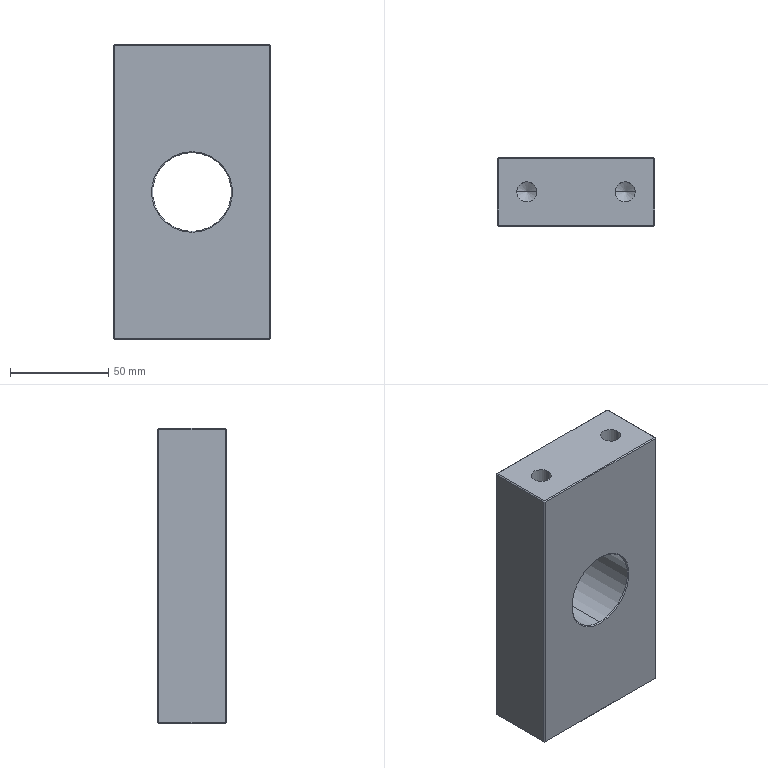Part | SolidWorks | features HoleWzd 2, Chamfer 1, Extrusion 1 | 1 solid | 48 faces | box 80 x 35 x 150 mm | volume 365960 mm3 | plane 26 | cone 12 | cylinder 10 | commonest cylinder face diameters 10.2 x8 40 x2
STEP:
#1=CARTESIAN_POINT('',(30.1,17.5,-45.75));
#2=VERTEX_POINT('',#1);
#3=CARTESIAN_POINT('',(19.9,17.5,-45.75));
#4=VERTEX_POINT('',#3);
#5=CARTESIAN_POINT('',(25.,17.5,-45.75));
#6=DIRECTION('',(0.,0.,-1.));
#7=DIRECTION('',(-1.,0.,0.));
#8=AXIS2_PLACEMENT_3D('',#5,#6,#7);
#9=CIRCLE('',#8,5.1);
#10=EDGE_CURVE('',#2,#4,#9,.T.);
#11=ORIENTED_EDGE('',*,*,#10,.F.);
#12=CARTESIAN_POINT('',(30.1,17.5,-75.));
#13=VERTEX_POINT('',#12);
#14=CARTESIAN_POINT('',(30.1,17.5,-75.));
#15=DIRECTION('',(0.,0.,-1.));
#16=VECTOR('',#15,1000.);
#17=LINE('',#14,#16);
#18=EDGE_CURVE('',#2,#13,#17,.T.);
#19=ORIENTED_EDGE('',*,*,#18,.T.);
#20=CARTESIAN_POINT('',(19.9,17.5,-75.));
#21=VERTEX_POINT('',#20);
#22=CARTESIAN_POINT('',(25.,17.5,-75.));
#23=DIRECTION('',(0.,0.,-1.));
#24=DIRECTION('',(-1.,0.,0.));
#25=AXIS2_PLACEMENT_3D('',#22,#23,#24);
#26=CIRCLE('',#25,5.1);
#27=EDGE_CURVE('',#13,#21,#26,.T.);
#28=ORIENTED_EDGE('',*,*,#27,.T.);
#29=CARTESIAN_POINT('',(19.9,17.5,-75.));
#30=DIRECTION('',(0.,0.,-1.));
#31=VECTOR('',#30,1000.);
#32=LINE('',#29,#31);
#33=EDGE_CURVE('',#4,#21,#32,.T.);
#34=ORIENTED_EDGE('',*,*,#33,.F.);
#35=EDGE_LOOP('',(#11,#19,#28,#34));
#36=FACE_OUTER_BOUND('',#35,.T.);
#37=CARTESIAN_POINT('',(25.,17.5,-75.));
#38=DIRECTION('',(0.,0.,-1.));
#39=DIRECTION('',(-1.,0.,0.));
#40=AXIS2_PLACEMENT_3D('',#37,#38,#39);
#41=CYLINDRICAL_SURFACE('',#40,5.1);
#42=ADVANCED_FACE('',(#36),#41,.F.);
#43=CARTESIAN_POINT('',(25.,17.5,-42.686));
#44=VERTEX_POINT('',#43);
#45=CARTESIAN_POINT('',(19.9,17.5,-45.75));
#46=DIRECTION('',(-0.8572,0.,-0.515));
#47=VECTOR('',#46,1000.);
#48=LINE('',#45,#47);
#49=EDGE_CURVE('',#44,#4,#48,.T.);
#50=ORIENTED_EDGE('',*,*,#49,.F.);
#51=CARTESIAN_POINT('',(30.1,17.5,-45.75));
#52=DIRECTION('',(0.8572,0.,-0.515));
#53=VECTOR('',#52,1000.);
#54=LINE('',#51,#53);
#55=EDGE_CURVE('',#44,#2,#54,.T.);
#56=ORIENTED_EDGE('',*,*,#55,.T.);
#57=ORIENTED_EDGE('',*,*,#10,.T.);
#58=EDGE_LOOP('',(#50,#56,#57));
#59=FACE_OUTER_BOUND('',#58,.T.);
#60=CARTESIAN_POINT('',(25.,17.5,-45.75));
#61=DIRECTION('',(0.,0.,-1.));
#62=DIRECTION('',(-1.,0.,0.));
#63=AXIS2_PLACEMENT_3D('',#60,#61,#62);
#64=CONICAL_SURFACE('',#63,5.1,1.03);
#65=ADVANCED_FACE('',(#59),#64,.F.);
#66=CARTESIAN_POINT('',(-19.9,17.5,-45.75));
#67=VERTEX_POINT('',#66);
#68=CARTESIAN_POINT('',(-30.1,17.5,-45.75));
#69=VERTEX_POINT('',#68);
#70=CARTESIAN_POINT('',(-25.,17.5,-45.75));
#71=DIRECTION('',(0.,0.,-1.));
#72=DIRECTION('',(-1.,0.,0.));
#73=AXIS2_PLACEMENT_3D('',#70,#71,#72);
#74=CIRCLE('',#73,5.1);
#75=EDGE_CURVE('',#67,#69,#74,.T.);
#76=ORIENTED_EDGE('',*,*,#75,.F.);
#77=CARTESIAN_POINT('',(-19.9,17.5,-75.));
#78=VERTEX_POINT('',#77);
#79=CARTESIAN_POINT('',(-19.9,17.5,-75.));
#80=DIRECTION('',(0.,0.,-1.));
#81=VECTOR('',#80,1000.);
#82=LINE('',#79,#81);
#83=EDGE_CURVE('',#67,#78,#82,.T.);
#84=ORIENTED_EDGE('',*,*,#83,.T.);
#85=CARTESIAN_POINT('',(-30.1,17.5,-75.));
#86=VERTEX_POINT('',#85);
#87=CARTESIAN_POINT('',(-25.,17.5,-75.));
#88=DIRECTION('',(0.,0.,-1.));
#89=DIRECTION('',(-1.,0.,0.));
#90=AXIS2_PLACEMENT_3D('',#87,#88,#89);
#91=CIRCLE('',#90,5.1);
#92=EDGE_CURVE('',#78,#86,#91,.T.);
#93=ORIENTED_EDGE('',*,*,#92,.T.);
#94=CARTESIAN_POINT('',(-30.1,17.5,-75.));
#95=DIRECTION('',(0.,0.,-1.));
#96=VECTOR('',#95,1000.);
#97=LINE('',#94,#96);
#98=EDGE_CURVE('',#69,#86,#97,.T.);
#99=ORIENTED_EDGE('',*,*,#98,.F.);
#100=EDGE_LOOP('',(#76,#84,#93,#99));
#101=FACE_OUTER_BOUND('',#100,.T.);
#102=CARTESIAN_POINT('',(-25.,17.5,-75.));
#103=DIRECTION('',(0.,0.,-1.));
#104=DIRECTION('',(-1.,0.,0.));
#105=AXIS2_PLACEMENT_3D('',#102,#103,#104);
#106=CYLINDRICAL_SURFACE('',#105,5.1);
#107=ADVANCED_FACE('',(#101),#106,.F.);
#108=CARTESIAN_POINT('',(-25.,17.5,-42.686));
#109=VERTEX_POINT('',#108);
#110=CARTESIAN_POINT('',(-30.1,17.5,-45.75));
#111=DIRECTION('',(-0.8572,0.,-0.515));
#112=VECTOR('',#111,1000.);
#113=LINE('',#110,#112);
#114=EDGE_CURVE('',#109,#69,#113,.T.);
#115=ORIENTED_EDGE('',*,*,#114,.F.);
#116=CARTESIAN_POINT('',(-19.9,17.5,-45.75));
#117=DIRECTION('',(0.8572,0.,-0.515));
#118=VECTOR('',#117,1000.);
#119=LINE('',#116,#118);
#120=EDGE_CURVE('',#109,#67,#119,.T.);
#121=ORIENTED_EDGE('',*,*,#120,.T.);
#122=ORIENTED_EDGE('',*,*,#75,.T.);
#123=EDGE_LOOP('',(#115,#121,#122));
#124=FACE_OUTER_BOUND('',#123,.T.);
#125=CARTESIAN_POINT('',(-25.,17.5,-45.75));
#126=DIRECTION('',(0.,0.,-1.));
#127=DIRECTION('',(-1.,0.,0.));
#128=AXIS2_PLACEMENT_3D('',#125,#126,#127);
#129=CONICAL_SURFACE('',#128,5.1,1.03);
#130=ADVANCED_FACE('',(#124),#129,.F.);
#131=CARTESIAN_POINT('',(19.9,17.5,45.75));
#132=VERTEX_POINT('',#131);
#133=CARTESIAN_POINT('',(30.1,17.5,45.75));
#134=VERTEX_POINT('',#133);
#135=CARTESIAN_POINT('',(25.,17.5,45.75));
#136=DIRECTION('',(0.,0.,1.));
#137=DIRECTION('',(1.,0.,0.));
#138=AXIS2_PLACEMENT_3D('',#135,#136,#137);
#139=CIRCLE('',#138,5.1);
#140=EDGE_CURVE('',#132,#134,#139,.T.);
#141=ORIENTED_EDGE('',*,*,#140,.F.);
#142=CARTESIAN_POINT('',(19.9,17.5,75.));
#143=VERTEX_POINT('',#142);
#144=CARTESIAN_POINT('',(19.9,17.5,75.));
#145=DIRECTION('',(0.,0.,1.));
#146=VECTOR('',#145,1000.);
#147=LINE('',#144,#146);
#148=EDGE_CURVE('',#132,#143,#147,.T.);
#149=ORIENTED_EDGE('',*,*,#148,.T.);
#150=CARTESIAN_POINT('',(30.1,17.5,75.));
#151=VERTEX_POINT('',#150);
#152=CARTESIAN_POINT('',(25.,17.5,75.));
#153=DIRECTION('',(0.,0.,1.));
#154=DIRECTION('',(1.,0.,0.));
#155=AXIS2_PLACEMENT_3D('',#152,#153,#154);
#156=CIRCLE('',#155,5.1);
#157=EDGE_CURVE('',#143,#151,#156,.T.);
#158=ORIENTED_EDGE('',*,*,#157,.T.);
#159=CARTESIAN_POINT('',(30.1,17.5,75.));
#160=DIRECTION('',(0.,0.,1.));
#161=VECTOR('',#160,1000.);
#162=LINE('',#159,#161);
#163=EDGE_CURVE('',#134,#151,#162,.T.);
#164=ORIENTED_EDGE('',*,*,#163,.F.);
#165=EDGE_LOOP('',(#141,#149,#158,#164));
#166=FACE_OUTER_BOUND('',#165,.T.);
#167=CARTESIAN_POINT('',(25.,17.5,75.));
#168=DIRECTION('',(0.,0.,1.));
#169=DIRECTION('',(1.,0.,0.));
#170=AXIS2_PLACEMENT_3D('',#167,#168,#169);
#171=CYLINDRICAL_SURFACE('',#170,5.1);
#172=ADVANCED_FACE('',(#166),#171,.F.);
#173=CARTESIAN_POINT('',(25.,17.5,42.686));
#174=VERTEX_POINT('',#173);
#175=CARTESIAN_POINT('',(30.1,17.5,45.75));
#176=DIRECTION('',(0.8572,0.,0.515));
#177=VECTOR('',#176,1000.);
#178=LINE('',#175,#177);
#179=EDGE_CURVE('',#174,#134,#178,.T.);
#180=ORIENTED_EDGE('',*,*,#179,.F.);
#181=CARTESIAN_POINT('',(19.9,17.5,45.75));
#182=DIRECTION('',(-0.8572,0.,0.515));
#183=VECTOR('',#182,1000.);
#184=LINE('',#181,#183);
#185=EDGE_CURVE('',#174,#132,#184,.T.);
#186=ORIENTED_EDGE('',*,*,#185,.T.);
#187=ORIENTED_EDGE('',*,*,#140,.T.);
#188=EDGE_LOOP('',(#180,#186,#187));
#189=FACE_OUTER_BOUND('',#188,.T.);
#190=CARTESIAN_POINT('',(25.,17.5,45.75));
#191=DIRECTION('',(0.,0.,1.));
#192=DIRECTION('',(1.,0.,0.));
#193=AXIS2_PLACEMENT_3D('',#190,#191,#192);
#194=CONICAL_SURFACE('',#193,5.1,1.03);
#195=ADVANCED_FACE('',(#189),#194,.F.);
#196=CARTESIAN_POINT('',(-30.1,17.5,45.75));
#197=VERTEX_POINT('',#196);
#198=CARTESIAN_POINT('',(-19.9,17.5,45.75));
#199=VERTEX_POINT('',#198);
#200=CARTESIAN_POINT('',(-25.,17.5,45.75));
#201=DIRECTION('',(0.,0.,1.));
#202=DIRECTION('',(1.,0.,0.));
#203=AXIS2_PLACEMENT_3D('',#200,#201,#202);
#204=CIRCLE('',#203,5.1);
#205=EDGE_CURVE('',#197,#199,#204,.T.);
#206=ORIENTED_EDGE('',*,*,#205,.F.);
#207=CARTESIAN_POINT('',(-30.1,17.5,75.));
#208=VERTEX_POINT('',#207);
#209=CARTESIAN_POINT('',(-30.1,17.5,75.));
#210=DIRECTION('',(0.,0.,1.));
#211=VECTOR('',#210,1000.);
#212=LINE('',#209,#211);
#213=EDGE_CURVE('',#197,#208,#212,.T.);
#214=ORIENTED_EDGE('',*,*,#213,.T.);
#215=CARTESIAN_POINT('',(-19.9,17.5,75.));
#216=VERTEX_POINT('',#215);
#217=CARTESIAN_POINT('',(-25.,17.5,75.));
#218=DIRECTION('',(0.,0.,1.));
#219=DIRECTION('',(1.,0.,0.));
#220=AXIS2_PLACEMENT_3D('',#217,#218,#219);
#221=CIRCLE('',#220,5.1);
#222=EDGE_CURVE('',#208,#216,#221,.T.);
#223=ORIENTED_EDGE('',*,*,#222,.T.);
#224=CARTESIAN_POINT('',(-19.9,17.5,75.));
#225=DIRECTION('',(0.,0.,1.));
#226=VECTOR('',#225,1000.);
#227=LINE('',#224,#226);
#228=EDGE_CURVE('',#199,#216,#227,.T.);
#229=ORIENTED_EDGE('',*,*,#228,.F.);
#230=EDGE_LOOP('',(#206,#214,#223,#229));
#231=FACE_OUTER_BOUND('',#230,.T.);
#232=CARTESIAN_POINT('',(-25.,17.5,75.));
#233=DIRECTION('',(0.,0.,1.));
#234=DIRECTION('',(1.,0.,0.));
#235=AXIS2_PLACEMENT_3D('',#232,#233,#234);
#236=CYLINDRICAL_SURFACE('',#235,5.1);
#237=ADVANCED_FACE('',(#231),#236,.F.);
#238=CARTESIAN_POINT('',(-25.,17.5,42.686));
#239=VERTEX_POINT('',#238);
#240=CARTESIAN_POINT('',(-19.9,17.5,45.75));
#241=DIRECTION('',(0.8572,0.,0.515));
#242=VECTOR('',#241,1000.);
#243=LINE('',#240,#242);
#244=EDGE_CURVE('',#239,#199,#243,.T.);
#245=ORIENTED_EDGE('',*,*,#244,.F.);
#246=CARTESIAN_POINT('',(-30.1,17.5,45.75));
#247=DIRECTION('',(-0.8572,0.,0.515));
#248=VECTOR('',#247,1000.);
#249=LINE('',#246,#248);
#250=EDGE_CURVE('',#239,#197,#249,.T.);
#251=ORIENTED_EDGE('',*,*,#250,.T.);
#252=ORIENTED_EDGE('',*,*,#205,.T.);
#253=EDGE_LOOP('',(#245,#251,#252));
#254=FACE_OUTER_BOUND('',#253,.T.);
#255=CARTESIAN_POINT('',(-25.,17.5,45.75));
#256=DIRECTION('',(0.,0.,1.));
#257=DIRECTION('',(1.,0.,0.));
#258=AXIS2_PLACEMENT_3D('',#255,#256,#257);
#259=CONICAL_SURFACE('',#258,5.1,1.03);
#260=ADVANCED_FACE('',(#254),#259,.F.);
#261=CARTESIAN_POINT('',(0.,34.5,-20.));
#262=VERTEX_POINT('',#261);
#263=CARTESIAN_POINT('',(0.,34.5,20.));
#264=VERTEX_POINT('',#263);
#265=CARTESIAN_POINT('',(0.,34.5,0.));
#266=DIRECTION('',(0.,1.,0.));
#267=DIRECTION('',(0.,0.,-1.));
#268=AXIS2_PLACEMENT_3D('',#265,#266,#267);
#269=CIRCLE('',#268,20.);
#270=EDGE_CURVE('',#262,#264,#269,.T.);
#271=ORIENTED_EDGE('',*,*,#270,.F.);
#272=CARTESIAN_POINT('',(0.,35.,-20.5));
#273=VERTEX_POINT('',#272);
#274=CARTESIAN_POINT('',(0.,34.5,-20.));
#275=DIRECTION('',(0.,0.7071,-0.7071));
#276=VECTOR('',#275,1000.);
#277=LINE('',#274,#276);
#278=EDGE_CURVE('',#262,#273,#277,.T.);
#279=ORIENTED_EDGE('',*,*,#278,.T.);
#280=CARTESIAN_POINT('',(0.,35.,20.5));
#281=VERTEX_POINT('',#280);
#282=CARTESIAN_POINT('',(0.,35.,0.));
#283=DIRECTION('',(0.,-1.,0.));
#284=DIRECTION('',(0.,0.,-1.));
#285=AXIS2_PLACEMENT_3D('',#282,#283,#284);
#286=CIRCLE('',#285,20.5);
#287=EDGE_CURVE('',#281,#273,#286,.T.);
#288=ORIENTED_EDGE('',*,*,#287,.F.);
#289=CARTESIAN_POINT('',(0.,34.5,20.));
#290=DIRECTION('',(0.,0.7071,0.7071));
#291=VECTOR('',#290,1000.);
#292=LINE('',#289,#291);
#293=EDGE_CURVE('',#264,#281,#292,.T.);
#294=ORIENTED_EDGE('',*,*,#293,.F.);
#295=EDGE_LOOP('',(#271,#279,#288,#294));
#296=FACE_OUTER_BOUND('',#295,.T.);
#297=CARTESIAN_POINT('',(0.,34.5,0.));
#298=DIRECTION('',(0.,1.,0.));
#299=DIRECTION('',(0.,0.,1.));
#300=AXIS2_PLACEMENT_3D('',#297,#298,#299);
#301=CONICAL_SURFACE('',#300,20.,0.7854);
#302=ADVANCED_FACE('',(#296),#301,.F.);
#303=CARTESIAN_POINT('',(0.,0.5,20.));
#304=VERTEX_POINT('',#303);
#305=CARTESIAN_POINT('',(0.,0.5,-20.));
#306=VERTEX_POINT('',#305);
#307=CARTESIAN_POINT('',(0.,0.5,0.));
#308=DIRECTION('',(0.,-1.,0.));
#309=DIRECTION('',(0.,0.,-1.));
#310=AXIS2_PLACEMENT_3D('',#307,#308,#309);
#311=CIRCLE('',#310,20.);
#312=EDGE_CURVE('',#304,#306,#311,.T.);
#313=ORIENTED_EDGE('',*,*,#312,.F.);
#314=CARTESIAN_POINT('',(0.,0.,20.5));
#315=VERTEX_POINT('',#314);
#316=CARTESIAN_POINT('',(0.,0.,20.5));
#317=DIRECTION('',(0.,-0.7071,0.7071));
#318=VECTOR('',#317,1000.);
#319=LINE('',#316,#318);
#320=EDGE_CURVE('',#304,#315,#319,.T.);
#321=ORIENTED_EDGE('',*,*,#320,.T.);
#322=CARTESIAN_POINT('',(0.,0.,-20.5));
#323=VERTEX_POINT('',#322);
#324=CARTESIAN_POINT('',(0.,0.,0.));
#325=DIRECTION('',(0.,1.,0.));
#326=DIRECTION('',(0.,0.,-1.));
#327=AXIS2_PLACEMENT_3D('',#324,#325,#326);
#328=CIRCLE('',#327,20.5);
#329=EDGE_CURVE('',#323,#315,#328,.T.);
#330=ORIENTED_EDGE('',*,*,#329,.F.);
#331=CARTESIAN_POINT('',(0.,0.,-20.5));
#332=DIRECTION('',(0.,-0.7071,-0.7071));
#333=VECTOR('',#332,1000.);
#334=LINE('',#331,#333);
#335=EDGE_CURVE('',#306,#323,#334,.T.);
#336=ORIENTED_EDGE('',*,*,#335,.F.);
#337=EDGE_LOOP('',(#313,#321,#330,#336));
#338=FACE_OUTER_BOUND('',#337,.T.);
#339=CARTESIAN_POINT('',(0.,0.,0.));
#340=DIRECTION('',(0.,-1.,0.));
#341=DIRECTION('',(0.,0.,-1.));
#342=AXIS2_PLACEMENT_3D('',#339,#340,#341);
#343=CONICAL_SURFACE('',#342,20.5,0.7854);
#344=ADVANCED_FACE('',(#338),#343,.F.);
#345=ORIENTED_EDGE('',*,*,#270,.T.);
#346=CARTESIAN_POINT('',(0.,35.,20.));
#347=DIRECTION('',(0.,-1.,0.));
#348=VECTOR('',#347,1000.);
#349=LINE('',#346,#348);
#350=EDGE_CURVE('',#264,#304,#349,.T.);
#351=ORIENTED_EDGE('',*,*,#350,.T.);
#352=ORIENTED_EDGE('',*,*,#312,.T.);
#353=CARTESIAN_POINT('',(0.,35.,-20.));
#354=DIRECTION('',(0.,-1.,0.));
#355=VECTOR('',#354,1000.);
#356=LINE('',#353,#355);
#357=EDGE_CURVE('',#262,#306,#356,.T.);
#358=ORIENTED_EDGE('',*,*,#357,.F.);
#359=EDGE_LOOP('',(#345,#351,#352,#358));
#360=FACE_OUTER_BOUND('',#359,.T.);
#361=CARTESIAN_POINT('',(0.,35.,0.));
#362=DIRECTION('',(0.,-1.,0.));
#363=DIRECTION('',(0.,0.,-1.));
#364=AXIS2_PLACEMENT_3D('',#361,#362,#363);
#365=CYLINDRICAL_SURFACE('',#364,20.);
#366=ADVANCED_FACE('',(#360),#365,.F.);
#367=ORIENTED_EDGE('',*,*,#287,.T.);
#368=CARTESIAN_POINT('',(0.,35.,0.));
#369=DIRECTION('',(0.,-1.,0.));
#370=DIRECTION('',(0.,0.,-1.));
#371=AXIS2_PLACEMENT_3D('',#368,#369,#370);
#372=CIRCLE('',#371,20.5);
#373=EDGE_CURVE('',#273,#281,#372,.T.);
#374=ORIENTED_EDGE('',*,*,#373,.T.);
#375=EDGE_LOOP('',(#367,#374));
#376=FACE_BOUND('',#375,.T.);
#377=CARTESIAN_POINT('',(-39.5,35.,-74.5));
#378=VERTEX_POINT('',#377);
#379=CARTESIAN_POINT('',(-39.5,35.,74.5));
#380=VERTEX_POINT('',#379);
#381=CARTESIAN_POINT('',(-39.5,35.,0.));
#382=DIRECTION('',(0.,0.,1.));
#383=VECTOR('',#382,1000.);
#384=LINE('',#381,#383);
#385=EDGE_CURVE('',#378,#380,#384,.T.);
#386=ORIENTED_EDGE('',*,*,#385,.T.);
#387=CARTESIAN_POINT('',(39.5,35.,74.5));
#388=VERTEX_POINT('',#387);
#389=CARTESIAN_POINT('',(0.,35.,74.5));
#390=DIRECTION('',(1.,0.,0.));
#391=VECTOR('',#390,1000.);
#392=LINE('',#389,#391);
#393=EDGE_CURVE('',#380,#388,#392,.T.);
#394=ORIENTED_EDGE('',*,*,#393,.T.);
#395=CARTESIAN_POINT('',(39.5,35.,-74.5));
#396=VERTEX_POINT('',#395);
#397=CARTESIAN_POINT('',(39.5,35.,0.));
#398=DIRECTION('',(0.,0.,-1.));
#399=VECTOR('',#398,1000.);
#400=LINE('',#397,#399);
#401=EDGE_CURVE('',#388,#396,#400,.T.);
#402=ORIENTED_EDGE('',*,*,#401,.T.);
#403=CARTESIAN_POINT('',(0.,35.,-74.5));
#404=DIRECTION('',(-1.,0.,0.));
#405=VECTOR('',#404,1000.);
#406=LINE('',#403,#405);
#407=EDGE_CURVE('',#396,#378,#406,.T.);
#408=ORIENTED_EDGE('',*,*,#407,.T.);
#409=EDGE_LOOP('',(#386,#394,#402,#408));
#410=FACE_OUTER_BOUND('',#409,.T.);
#411=CARTESIAN_POINT('',(0.,35.,0.));
#412=DIRECTION('',(0.,-1.,0.));
#413=DIRECTION('',(0.,0.,-1.));
#414=AXIS2_PLACEMENT_3D('',#411,#412,#413);
#415=PLANE('',#414);
#416=ADVANCED_FACE('',(#376,#410),#415,.F.);
#417=ORIENTED_EDGE('',*,*,#329,.T.);
#418=CARTESIAN_POINT('',(0.,0.,0.));
#419=DIRECTION('',(0.,1.,0.));
#420=DIRECTION('',(0.,0.,-1.));
#421=AXIS2_PLACEMENT_3D('',#418,#419,#420);
#422=CIRCLE('',#421,20.5);
#423=EDGE_CURVE('',#315,#323,#422,.T.);
#424=ORIENTED_EDGE('',*,*,#423,.T.);
#425=EDGE_LOOP('',(#417,#424));
#426=FACE_BOUND('',#425,.T.);
#427=CARTESIAN_POINT('',(39.5,0.,-74.5));
#428=VERTEX_POINT('',#427);
#429=CARTESIAN_POINT('',(39.5,0.,74.5));
#430=VERTEX_POINT('',#429);
#431=CARTESIAN_POINT('',(39.5,0.,75.));
#432=DIRECTION('',(0.,0.,1.));
#433=VECTOR('',#432,1000.);
#434=LINE('',#431,#433);
#435=EDGE_CURVE('',#428,#430,#434,.T.);
#436=ORIENTED_EDGE('',*,*,#435,.T.);
#437=CARTESIAN_POINT('',(-39.5,0.,74.5));
#438=VERTEX_POINT('',#437);
#439=CARTESIAN_POINT('',(-40.,0.,74.5));
#440=DIRECTION('',(-1.,0.,0.));
#441=VECTOR('',#440,1000.);
#442=LINE('',#439,#441);
#443=EDGE_CURVE('',#430,#438,#442,.T.);
#444=ORIENTED_EDGE('',*,*,#443,.T.);
#445=CARTESIAN_POINT('',(-39.5,0.,-74.5));
#446=VERTEX_POINT('',#445);
#447=CARTESIAN_POINT('',(-39.5,0.,-75.));
#448=DIRECTION('',(0.,0.,-1.));
#449=VECTOR('',#448,1000.);
#450=LINE('',#447,#449);
#451=EDGE_CURVE('',#438,#446,#450,.T.);
#452=ORIENTED_EDGE('',*,*,#451,.T.);
#453=CARTESIAN_POINT('',(40.,0.,-74.5));
#454=DIRECTION('',(1.,0.,0.));
#455=VECTOR('',#454,1000.);
#456=LINE('',#453,#455);
#457=EDGE_CURVE('',#446,#428,#456,.T.);
#458=ORIENTED_EDGE('',*,*,#457,.T.);
#459=EDGE_LOOP('',(#436,#444,#452,#458));
#460=FACE_OUTER_BOUND('',#459,.T.);
#461=CARTESIAN_POINT('',(0.,0.,0.));
#462=DIRECTION('',(0.,-1.,0.));
#463=DIRECTION('',(0.,0.,-1.));
#464=AXIS2_PLACEMENT_3D('',#461,#462,#463);
#465=PLANE('',#464);
#466=ADVANCED_FACE('',(#426,#460),#465,.T.);
#467=CARTESIAN_POINT('',(40.,0.5,74.5));
#468=VERTEX_POINT('',#467);
#469=CARTESIAN_POINT('',(40.,0.5,-74.5));
#470=VERTEX_POINT('',#469);
#471=CARTESIAN_POINT('',(40.,0.5,-75.));
#472=DIRECTION('',(0.,0.,-1.));
#473=VECTOR('',#472,1000.);
#474=LINE('',#471,#473);
#475=EDGE_CURVE('',#468,#470,#474,.T.);
#476=ORIENTED_EDGE('',*,*,#475,.T.);
#477=CARTESIAN_POINT('',(40.,34.5,-74.5));
#478=VERTEX_POINT('',#477);
#479=CARTESIAN_POINT('',(40.,35.,-74.5));
#480=DIRECTION('',(0.,1.,0.));
#481=VECTOR('',#480,1000.);
#482=LINE('',#479,#481);
#483=EDGE_CURVE('',#470,#478,#482,.T.);
#484=ORIENTED_EDGE('',*,*,#483,.T.);
#485=CARTESIAN_POINT('',(40.,34.5,74.5));
#486=VERTEX_POINT('',#485);
#487=CARTESIAN_POINT('',(40.,34.5,75.));
#488=DIRECTION('',(0.,0.,1.));
#489=VECTOR('',#488,1000.);
#490=LINE('',#487,#489);
#491=EDGE_CURVE('',#478,#486,#490,.T.);
#492=ORIENTED_EDGE('',*,*,#491,.T.);
#493=CARTESIAN_POINT('',(40.,35.,74.5));
#494=DIRECTION('',(0.,-1.,0.));
#495=VECTOR('',#494,1000.);
#496=LINE('',#493,#495);
#497=EDGE_CURVE('',#486,#468,#496,.T.);
#498=ORIENTED_EDGE('',*,*,#497,.T.);
#499=EDGE_LOOP('',(#476,#484,#492,#498));
#500=FACE_OUTER_BOUND('',#499,.T.);
#501=CARTESIAN_POINT('',(40.,35.,75.));
#502=DIRECTION('',(-1.,0.,0.));
#503=DIRECTION('',(0.,0.,1.));
#504=AXIS2_PLACEMENT_3D('',#501,#502,#503);
#505=PLANE('',#504);
#506=ADVANCED_FACE('',(#500),#505,.F.);
#507=CARTESIAN_POINT('',(25.,17.5,-75.));
#508=DIRECTION('',(0.,0.,-1.));
#509=DIRECTION('',(-1.,0.,0.));
#510=AXIS2_PLACEMENT_3D('',#507,#508,#509);
#511=CIRCLE('',#510,5.1);
#512=EDGE_CURVE('',#21,#13,#511,.T.);
#513=ORIENTED_EDGE('',*,*,#512,.F.);
#514=ORIENTED_EDGE('',*,*,#27,.F.);
#515=EDGE_LOOP('',(#513,#514));
#516=FACE_BOUND('',#515,.T.);
#517=CARTESIAN_POINT('',(-25.,17.5,-75.));
#518=DIRECTION('',(0.,0.,-1.));
#519=DIRECTION('',(-1.,0.,0.));
#520=AXIS2_PLACEMENT_3D('',#517,#518,#519);
#521=CIRCLE('',#520,5.1);
#522=EDGE_CURVE('',#86,#78,#521,.T.);
#523=ORIENTED_EDGE('',*,*,#522,.F.);
#524=ORIENTED_EDGE('',*,*,#92,.F.);
#525=EDGE_LOOP('',(#523,#524));
#526=FACE_BOUND('',#525,.T.);
#527=CARTESIAN_POINT('',(-39.5,0.5,-75.));
#528=VERTEX_POINT('',#527);
#529=CARTESIAN_POINT('',(-39.5,34.5,-75.));
#530=VERTEX_POINT('',#529);
#531=CARTESIAN_POINT('',(-39.5,35.,-75.));
#532=DIRECTION('',(0.,1.,0.));
#533=VECTOR('',#532,1000.);
#534=LINE('',#531,#533);
#535=EDGE_CURVE('',#528,#530,#534,.T.);
#536=ORIENTED_EDGE('',*,*,#535,.T.);
#537=CARTESIAN_POINT('',(39.5,34.5,-75.));
#538=VERTEX_POINT('',#537);
#539=CARTESIAN_POINT('',(-40.,34.5,-75.));
#540=DIRECTION('',(1.,0.,0.));
#541=VECTOR('',#540,1000.);
#542=LINE('',#539,#541);
#543=EDGE_CURVE('',#530,#538,#542,.T.);
#544=ORIENTED_EDGE('',*,*,#543,.T.);
#545=CARTESIAN_POINT('',(39.5,0.5,-75.));
#546=VERTEX_POINT('',#545);
#547=CARTESIAN_POINT('',(39.5,35.,-75.));
#548=DIRECTION('',(0.,-1.,0.));
#549=VECTOR('',#548,1000.);
#550=LINE('',#547,#549);
#551=EDGE_CURVE('',#538,#546,#550,.T.);
#552=ORIENTED_EDGE('',*,*,#551,.T.);
#553=CARTESIAN_POINT('',(-40.,0.5,-75.));
#554=DIRECTION('',(-1.,0.,0.));
#555=VECTOR('',#554,1000.);
#556=LINE('',#553,#555);
#557=EDGE_CURVE('',#546,#528,#556,.T.);
#558=ORIENTED_EDGE('',*,*,#557,.T.);
#559=EDGE_LOOP('',(#536,#544,#552,#558));
#560=FACE_OUTER_BOUND('',#559,.T.);
#561=CARTESIAN_POINT('',(-40.,35.,-75.));
#562=DIRECTION('',(0.,0.,1.));
#563=DIRECTION('',(1.,0.,0.));
#564=AXIS2_PLACEMENT_3D('',#561,#562,#563);
#565=PLANE('',#564);
#566=ADVANCED_FACE('',(#516,#526,#560),#565,.F.);
#567=CARTESIAN_POINT('',(-40.,0.5,74.5));
#568=VERTEX_POINT('',#567);
#569=CARTESIAN_POINT('',(-40.,34.5,74.5));
#570=VERTEX_POINT('',#569);
#571=CARTESIAN_POINT('',(-40.,35.,74.5));
#572=DIRECTION('',(0.,1.,0.));
#573=VECTOR('',#572,1000.);
#574=LINE('',#571,#573);
#575=EDGE_CURVE('',#568,#570,#574,.T.);
#576=ORIENTED_EDGE('',*,*,#575,.T.);
#577=CARTESIAN_POINT('',(-40.,34.5,-74.5));
#578=VERTEX_POINT('',#577);
#579=CARTESIAN_POINT('',(-40.,34.5,75.));
#580=DIRECTION('',(0.,0.,-1.));
#581=VECTOR('',#580,1000.);
#582=LINE('',#579,#581);
#583=EDGE_CURVE('',#570,#578,#582,.T.);
#584=ORIENTED_EDGE('',*,*,#583,.T.);
#585=CARTESIAN_POINT('',(-40.,0.5,-74.5));
#586=VERTEX_POINT('',#585);
#587=CARTESIAN_POINT('',(-40.,35.,-74.5));
#588=DIRECTION('',(0.,-1.,0.));
#589=VECTOR('',#588,1000.);
#590=LINE('',#587,#589);
#591=EDGE_CURVE('',#578,#586,#590,.T.);
#592=ORIENTED_EDGE('',*,*,#591,.T.);
#593=CARTESIAN_POINT('',(-40.,0.5,75.));
#594=DIRECTION('',(0.,0.,1.));
#595=VECTOR('',#594,1000.);
#596=LINE('',#593,#595);
#597=EDGE_CURVE('',#586,#568,#596,.T.);
#598=ORIENTED_EDGE('',*,*,#597,.T.);
#599=EDGE_LOOP('',(#576,#584,#592,#598));
#600=FACE_OUTER_BOUND('',#599,.T.);
#601=CARTESIAN_POINT('',(-40.,35.,75.));
#602=DIRECTION('',(1.,0.,0.));
#603=DIRECTION('',(0.,0.,-1.));
#604=AXIS2_PLACEMENT_3D('',#601,#602,#603);
#605=PLANE('',#604);
#606=ADVANCED_FACE('',(#600),#605,.F.);
#607=CARTESIAN_POINT('',(25.,17.5,75.));
#608=DIRECTION('',(0.,0.,1.));
#609=DIRECTION('',(1.,0.,0.));
#610=AXIS2_PLACEMENT_3D('',#607,#608,#609);
#611=CIRCLE('',#610,5.1);
#612=EDGE_CURVE('',#151,#143,#611,.T.);
#613=ORIENTED_EDGE('',*,*,#612,.F.);
#614=ORIENTED_EDGE('',*,*,#157,.F.);
#615=EDGE_LOOP('',(#613,#614));
#616=FACE_BOUND('',#615,.T.);
#617=CARTESIAN_POINT('',(-25.,17.5,75.));
#618=DIRECTION('',(0.,0.,1.));
#619=DIRECTION('',(1.,0.,0.));
#620=AXIS2_PLACEMENT_3D('',#617,#618,#619);
#621=CIRCLE('',#620,5.1);
#622=EDGE_CURVE('',#216,#208,#621,.T.);
#623=ORIENTED_EDGE('',*,*,#622,.F.);
#624=ORIENTED_EDGE('',*,*,#222,.F.);
#625=EDGE_LOOP('',(#623,#624));
#626=FACE_BOUND('',#625,.T.);
#627=CARTESIAN_POINT('',(39.5,34.5,75.));
#628=VERTEX_POINT('',#627);
#629=CARTESIAN_POINT('',(-39.5,34.5,75.));
#630=VERTEX_POINT('',#629);
#631=CARTESIAN_POINT('',(-40.,34.5,75.));
#632=DIRECTION('',(-1.,0.,0.));
#633=VECTOR('',#632,1000.);
#634=LINE('',#631,#633);
#635=EDGE_CURVE('',#628,#630,#634,.T.);
#636=ORIENTED_EDGE('',*,*,#635,.T.);
#637=CARTESIAN_POINT('',(-39.5,0.5,75.));
#638=VERTEX_POINT('',#637);
#639=CARTESIAN_POINT('',(-39.5,35.,75.));
#640=DIRECTION('',(0.,-1.,0.));
#641=VECTOR('',#640,1000.);
#642=LINE('',#639,#641);
#643=EDGE_CURVE('',#630,#638,#642,.T.);
#644=ORIENTED_EDGE('',*,*,#643,.T.);
#645=CARTESIAN_POINT('',(39.5,0.5,75.));
#646=VERTEX_POINT('',#645);
#647=CARTESIAN_POINT('',(40.,0.5,75.));
#648=DIRECTION('',(1.,0.,0.));
#649=VECTOR('',#648,1000.);
#650=LINE('',#647,#649);
#651=EDGE_CURVE('',#638,#646,#650,.T.);
#652=ORIENTED_EDGE('',*,*,#651,.T.);
#653=CARTESIAN_POINT('',(39.5,35.,75.));
#654=DIRECTION('',(0.,1.,0.));
#655=VECTOR('',#654,1000.);
#656=LINE('',#653,#655);
#657=EDGE_CURVE('',#646,#628,#656,.T.);
#658=ORIENTED_EDGE('',*,*,#657,.T.);
#659=EDGE_LOOP('',(#636,#644,#652,#658));
#660=FACE_OUTER_BOUND('',#659,.T.);
#661=CARTESIAN_POINT('',(-40.,35.,75.));
#662=DIRECTION('',(0.,0.,-1.));
#663=DIRECTION('',(-1.,0.,0.));
#664=AXIS2_PLACEMENT_3D('',#661,#662,#663);
#665=PLANE('',#664);
#666=ADVANCED_FACE('',(#616,#626,#660),#665,.F.);
#667=ORIENTED_EDGE('',*,*,#350,.F.);
#668=CARTESIAN_POINT('',(0.,34.5,0.));
#669=DIRECTION('',(0.,1.,0.));
#670=DIRECTION('',(0.,0.,-1.));
#671=AXIS2_PLACEMENT_3D('',#668,#669,#670);
#672=CIRCLE('',#671,20.);
#673=EDGE_CURVE('',#264,#262,#672,.T.);
#674=ORIENTED_EDGE('',*,*,#673,.T.);
#675=ORIENTED_EDGE('',*,*,#357,.T.);
#676=CARTESIAN_POINT('',(0.,0.5,0.));
#677=DIRECTION('',(0.,-1.,0.));
#678=DIRECTION('',(0.,0.,-1.));
#679=AXIS2_PLACEMENT_3D('',#676,#677,#678);
#680=CIRCLE('',#679,20.);
#681=EDGE_CURVE('',#306,#304,#680,.T.);
#682=ORIENTED_EDGE('',*,*,#681,.T.);
#683=EDGE_LOOP('',(#667,#674,#675,#682));
#684=FACE_OUTER_BOUND('',#683,.T.);
#685=CARTESIAN_POINT('',(0.,35.,0.));
#686=DIRECTION('',(0.,-1.,0.));
#687=DIRECTION('',(0.,0.,-1.));
#688=AXIS2_PLACEMENT_3D('',#685,#686,#687);
#689=CYLINDRICAL_SURFACE('',#688,20.);
#690=ADVANCED_FACE('',(#684),#689,.F.);
#691=ORIENTED_EDGE('',*,*,#320,.F.);
#692=ORIENTED_EDGE('',*,*,#681,.F.);
#693=ORIENTED_EDGE('',*,*,#335,.T.);
#694=ORIENTED_EDGE('',*,*,#423,.F.);
#695=EDGE_LOOP('',(#691,#692,#693,#694));
#696=FACE_OUTER_BOUND('',#695,.T.);
#697=CARTESIAN_POINT('',(0.,0.,0.));
#698=DIRECTION('',(0.,-1.,0.));
#699=DIRECTION('',(0.,0.,-1.));
#700=AXIS2_PLACEMENT_3D('',#697,#698,#699);
#701=CONICAL_SURFACE('',#700,20.5,0.7854);
#702=ADVANCED_FACE('',(#696),#701,.F.);
#703=ORIENTED_EDGE('',*,*,#278,.F.);
#704=ORIENTED_EDGE('',*,*,#673,.F.);
#705=ORIENTED_EDGE('',*,*,#293,.T.);
#706=ORIENTED_EDGE('',*,*,#373,.F.);
#707=EDGE_LOOP('',(#703,#704,#705,#706));
#708=FACE_OUTER_BOUND('',#707,.T.);
#709=CARTESIAN_POINT('',(0.,34.5,0.));
#710=DIRECTION('',(0.,1.,0.));
#711=DIRECTION('',(0.,0.,1.));
#712=AXIS2_PLACEMENT_3D('',#709,#710,#711);
#713=CONICAL_SURFACE('',#712,20.,0.7854);
#714=ADVANCED_FACE('',(#708),#713,.F.);
#715=CARTESIAN_POINT('',(-40.,34.5,74.5));
#716=DIRECTION('',(0.7071,0.,0.7071));
#717=VECTOR('',#716,1000.);
#718=LINE('',#715,#717);
#719=EDGE_CURVE('',#570,#630,#718,.T.);
#720=ORIENTED_EDGE('',*,*,#719,.F.);
#721=ORIENTED_EDGE('',*,*,#575,.F.);
#722=CARTESIAN_POINT('',(-39.5,0.5,75.));
#723=DIRECTION('',(-0.7071,0.,-0.7071));
#724=VECTOR('',#723,1000.);
#725=LINE('',#722,#724);
#726=EDGE_CURVE('',#638,#568,#725,.T.);
#727=ORIENTED_EDGE('',*,*,#726,.F.);
#728=ORIENTED_EDGE('',*,*,#643,.F.);
#729=EDGE_LOOP('',(#720,#721,#727,#728));
#730=FACE_OUTER_BOUND('',#729,.T.);
#731=CARTESIAN_POINT('',(-39.5,35.,75.));
#732=DIRECTION('',(0.7071,0.,-0.7071));
#733=DIRECTION('',(0.,-1.,0.));
#734=AXIS2_PLACEMENT_3D('',#731,#732,#733);
#735=PLANE('',#734);
#736=ADVANCED_FACE('',(#730),#735,.F.);
#737=CARTESIAN_POINT('',(-40.,34.5,74.5));
#738=DIRECTION('',(0.7071,0.7071,0.));
#739=VECTOR('',#738,1000.);
#740=LINE('',#737,#739);
#741=EDGE_CURVE('',#570,#380,#740,.T.);
#742=ORIENTED_EDGE('',*,*,#741,.F.);
#743=ORIENTED_EDGE('',*,*,#719,.T.);
#744=CARTESIAN_POINT('',(-39.5,34.75,74.75));
#745=DIRECTION('',(0.,-0.7071,0.7071));
#746=VECTOR('',#745,1000.);
#747=LINE('',#744,#746);
#748=EDGE_CURVE('',#380,#630,#747,.T.);
#749=ORIENTED_EDGE('',*,*,#748,.F.);
#750=EDGE_LOOP('',(#742,#743,#749));
#751=FACE_OUTER_BOUND('',#750,.T.);
#752=CARTESIAN_POINT('',(-40.,34.5,74.5));
#753=DIRECTION('',(-0.5774,0.5774,0.5774));
#754=DIRECTION('',(0.7071,0.,0.7071));
#755=AXIS2_PLACEMENT_3D('',#752,#753,#754);
#756=PLANE('',#755);
#757=ADVANCED_FACE('',(#751),#756,.T.);
#758=CARTESIAN_POINT('',(-39.5,0.5,75.));
#759=DIRECTION('',(0.,-0.7071,-0.7071));
#760=VECTOR('',#759,1000.);
#761=LINE('',#758,#760);
#762=EDGE_CURVE('',#638,#438,#761,.T.);
#763=ORIENTED_EDGE('',*,*,#762,.F.);
#764=ORIENTED_EDGE('',*,*,#726,.T.);
#765=CARTESIAN_POINT('',(-39.75,0.25,74.5));
#766=DIRECTION('',(-0.7071,0.7071,0.));
#767=VECTOR('',#766,1000.);
#768=LINE('',#765,#767);
#769=EDGE_CURVE('',#438,#568,#768,.T.);
#770=ORIENTED_EDGE('',*,*,#769,.F.);
#771=EDGE_LOOP('',(#763,#764,#770));
#772=FACE_OUTER_BOUND('',#771,.T.);
#773=CARTESIAN_POINT('',(-39.5,0.5,75.));
#774=DIRECTION('',(-0.5774,-0.5774,0.5774));
#775=DIRECTION('',(0.7071,0.,0.7071));
#776=AXIS2_PLACEMENT_3D('',#773,#774,#775);
#777=PLANE('',#776);
#778=ADVANCED_FACE('',(#772),#777,.T.);
#779=ORIENTED_EDGE('',*,*,#748,.T.);
#780=ORIENTED_EDGE('',*,*,#635,.F.);
#781=CARTESIAN_POINT('',(39.5,35.,74.5));
#782=DIRECTION('',(0.,-0.7071,0.7071));
#783=VECTOR('',#782,1000.);
#784=LINE('',#781,#783);
#785=EDGE_CURVE('',#388,#628,#784,.T.);
#786=ORIENTED_EDGE('',*,*,#785,.F.);
#787=ORIENTED_EDGE('',*,*,#393,.F.);
#788=EDGE_LOOP('',(#779,#780,#786,#787));
#789=FACE_OUTER_BOUND('',#788,.T.);
#790=CARTESIAN_POINT('',(0.,35.,74.5));
#791=DIRECTION('',(0.,-0.7071,-0.7071));
#792=DIRECTION('',(1.,0.,0.));
#793=AXIS2_PLACEMENT_3D('',#790,#791,#792);
#794=PLANE('',#793);
#795=ADVANCED_FACE('',(#789),#794,.F.);
#796=ORIENTED_EDGE('',*,*,#741,.T.);
#797=ORIENTED_EDGE('',*,*,#385,.F.);
#798=CARTESIAN_POINT('',(-39.75,34.75,-74.5));
#799=DIRECTION('',(0.7071,0.7071,0.));
#800=VECTOR('',#799,1000.);
#801=LINE('',#798,#800);
#802=EDGE_CURVE('',#578,#378,#801,.T.);
#803=ORIENTED_EDGE('',*,*,#802,.F.);
#804=ORIENTED_EDGE('',*,*,#583,.F.);
#805=EDGE_LOOP('',(#796,#797,#803,#804));
#806=FACE_OUTER_BOUND('',#805,.T.);
#807=CARTESIAN_POINT('',(-39.5,35.,0.));
#808=DIRECTION('',(0.7071,-0.7071,0.));
#809=DIRECTION('',(0.,0.,1.));
#810=AXIS2_PLACEMENT_3D('',#807,#808,#809);
#811=PLANE('',#810);
#812=ADVANCED_FACE('',(#806),#811,.F.);
#813=CARTESIAN_POINT('',(-40.,0.5,-74.5));
#814=DIRECTION('',(0.7071,0.,-0.7071));
#815=VECTOR('',#814,1000.);
#816=LINE('',#813,#815);
#817=EDGE_CURVE('',#586,#528,#816,.T.);
#818=ORIENTED_EDGE('',*,*,#817,.F.);
#819=ORIENTED_EDGE('',*,*,#591,.F.);
#820=CARTESIAN_POINT('',(-39.5,34.5,-75.));
#821=DIRECTION('',(-0.7071,0.,0.7071));
#822=VECTOR('',#821,1000.);
#823=LINE('',#820,#822);
#824=EDGE_CURVE('',#530,#578,#823,.T.);
#825=ORIENTED_EDGE('',*,*,#824,.F.);
#826=ORIENTED_EDGE('',*,*,#535,.F.);
#827=EDGE_LOOP('',(#818,#819,#825,#826));
#828=FACE_OUTER_BOUND('',#827,.T.);
#829=CARTESIAN_POINT('',(-40.,35.,-74.5));
#830=DIRECTION('',(0.7071,0.,0.7071));
#831=DIRECTION('',(0.,-1.,0.));
#832=AXIS2_PLACEMENT_3D('',#829,#830,#831);
#833=PLANE('',#832);
#834=ADVANCED_FACE('',(#828),#833,.F.);
#835=ORIENTED_EDGE('',*,*,#769,.T.);
#836=ORIENTED_EDGE('',*,*,#597,.F.);
#837=CARTESIAN_POINT('',(-40.,0.5,-74.5));
#838=DIRECTION('',(-0.7071,0.7071,0.));
#839=VECTOR('',#838,1000.);
#840=LINE('',#837,#839);
#841=EDGE_CURVE('',#446,#586,#840,.T.);
#842=ORIENTED_EDGE('',*,*,#841,.F.);
#843=ORIENTED_EDGE('',*,*,#451,.F.);
#844=EDGE_LOOP('',(#835,#836,#842,#843));
#845=FACE_OUTER_BOUND('',#844,.T.);
#846=CARTESIAN_POINT('',(-40.,0.5,75.));
#847=DIRECTION('',(-0.7071,-0.7071,0.));
#848=DIRECTION('',(0.,0.,-1.));
#849=AXIS2_PLACEMENT_3D('',#846,#847,#848);
#850=PLANE('',#849);
#851=ADVANCED_FACE('',(#845),#850,.T.);
#852=ORIENTED_EDGE('',*,*,#762,.T.);
#853=ORIENTED_EDGE('',*,*,#443,.F.);
#854=CARTESIAN_POINT('',(39.5,0.25,74.75));
#855=DIRECTION('',(0.,-0.7071,-0.7071));
#856=VECTOR('',#855,1000.);
#857=LINE('',#854,#856);
#858=EDGE_CURVE('',#646,#430,#857,.T.);
#859=ORIENTED_EDGE('',*,*,#858,.F.);
#860=ORIENTED_EDGE('',*,*,#651,.F.);
#861=EDGE_LOOP('',(#852,#853,#859,#860));
#862=FACE_OUTER_BOUND('',#861,.T.);
#863=CARTESIAN_POINT('',(-40.,0.5,75.));
#864=DIRECTION('',(0.,-0.7071,0.7071));
#865=DIRECTION('',(-1.,0.,0.));
#866=AXIS2_PLACEMENT_3D('',#863,#864,#865);
#867=PLANE('',#866);
#868=ADVANCED_FACE('',(#862),#867,.T.);
#869=CARTESIAN_POINT('',(39.75,34.5,74.75));
#870=DIRECTION('',(0.7071,0.,-0.7071));
#871=VECTOR('',#870,1000.);
#872=LINE('',#869,#871);
#873=EDGE_CURVE('',#628,#486,#872,.T.);
#874=ORIENTED_EDGE('',*,*,#873,.F.);
#875=ORIENTED_EDGE('',*,*,#657,.F.);
#876=CARTESIAN_POINT('',(40.,0.5,74.5));
#877=DIRECTION('',(-0.7071,0.,0.7071));
#878=VECTOR('',#877,1000.);
#879=LINE('',#876,#878);
#880=EDGE_CURVE('',#468,#646,#879,.T.);
#881=ORIENTED_EDGE('',*,*,#880,.F.);
#882=ORIENTED_EDGE('',*,*,#497,.F.);
#883=EDGE_LOOP('',(#874,#875,#881,#882));
#884=FACE_OUTER_BOUND('',#883,.T.);
#885=CARTESIAN_POINT('',(40.,35.,74.5));
#886=DIRECTION('',(-0.7071,0.,-0.7071));
#887=DIRECTION('',(0.,-1.,0.));
#888=AXIS2_PLACEMENT_3D('',#885,#886,#887);
#889=PLANE('',#888);
#890=ADVANCED_FACE('',(#884),#889,.F.);
#891=ORIENTED_EDGE('',*,*,#785,.T.);
#892=ORIENTED_EDGE('',*,*,#873,.T.);
#893=CARTESIAN_POINT('',(39.5,35.,74.5));
#894=DIRECTION('',(0.7071,-0.7071,0.));
#895=VECTOR('',#894,1000.);
#896=LINE('',#893,#895);
#897=EDGE_CURVE('',#388,#486,#896,.T.);
#898=ORIENTED_EDGE('',*,*,#897,.F.);
#899=EDGE_LOOP('',(#891,#892,#898));
#900=FACE_OUTER_BOUND('',#899,.T.);
#901=CARTESIAN_POINT('',(39.5,35.,74.5));
#902=DIRECTION('',(0.5774,0.5774,0.5774));
#903=DIRECTION('',(0.7071,0.,-0.7071));
#904=AXIS2_PLACEMENT_3D('',#901,#902,#903);
#905=PLANE('',#904);
#906=ADVANCED_FACE('',(#900),#905,.T.);
#907=ORIENTED_EDGE('',*,*,#824,.T.);
#908=ORIENTED_EDGE('',*,*,#802,.T.);
#909=CARTESIAN_POINT('',(-39.5,34.5,-75.));
#910=DIRECTION('',(0.,0.7071,0.7071));
#911=VECTOR('',#910,1000.);
#912=LINE('',#909,#911);
#913=EDGE_CURVE('',#530,#378,#912,.T.);
#914=ORIENTED_EDGE('',*,*,#913,.F.);
#915=EDGE_LOOP('',(#907,#908,#914));
#916=FACE_OUTER_BOUND('',#915,.T.);
#917=CARTESIAN_POINT('',(-39.5,34.5,-75.));
#918=DIRECTION('',(-0.5774,0.5774,-0.5774));
#919=DIRECTION('',(-0.7071,0.,0.7071));
#920=AXIS2_PLACEMENT_3D('',#917,#918,#919);
#921=PLANE('',#920);
#922=ADVANCED_FACE('',(#916),#921,.T.);
#923=ORIENTED_EDGE('',*,*,#841,.T.);
#924=ORIENTED_EDGE('',*,*,#817,.T.);
#925=CARTESIAN_POINT('',(-39.5,0.25,-74.75));
#926=DIRECTION('',(0.,0.7071,-0.7071));
#927=VECTOR('',#926,1000.);
#928=LINE('',#925,#927);
#929=EDGE_CURVE('',#446,#528,#928,.T.);
#930=ORIENTED_EDGE('',*,*,#929,.F.);
#931=EDGE_LOOP('',(#923,#924,#930));
#932=FACE_OUTER_BOUND('',#931,.T.);
#933=CARTESIAN_POINT('',(-40.,0.5,-74.5));
#934=DIRECTION('',(-0.5774,-0.5774,-0.5774));
#935=DIRECTION('',(-0.7071,0.,0.7071));
#936=AXIS2_PLACEMENT_3D('',#933,#934,#935);
#937=PLANE('',#936);
#938=ADVANCED_FACE('',(#932),#937,.T.);
#939=ORIENTED_EDGE('',*,*,#880,.T.);
#940=ORIENTED_EDGE('',*,*,#858,.T.);
#941=CARTESIAN_POINT('',(40.,0.5,74.5));
#942=DIRECTION('',(-0.7071,-0.7071,0.));
#943=VECTOR('',#942,1000.);
#944=LINE('',#941,#943);
#945=EDGE_CURVE('',#468,#430,#944,.T.);
#946=ORIENTED_EDGE('',*,*,#945,.F.);
#947=EDGE_LOOP('',(#939,#940,#946));
#948=FACE_OUTER_BOUND('',#947,.T.);
#949=CARTESIAN_POINT('',(40.,0.5,74.5));
#950=DIRECTION('',(0.5774,-0.5774,0.5774));
#951=DIRECTION('',(0.7071,0.,-0.7071));
#952=AXIS2_PLACEMENT_3D('',#949,#950,#951);
#953=PLANE('',#952);
#954=ADVANCED_FACE('',(#948),#953,.T.);
#955=ORIENTED_EDGE('',*,*,#897,.T.);
#956=ORIENTED_EDGE('',*,*,#491,.F.);
#957=CARTESIAN_POINT('',(40.,34.5,-74.5));
#958=DIRECTION('',(0.7071,-0.7071,0.));
#959=VECTOR('',#958,1000.);
#960=LINE('',#957,#959);
#961=EDGE_CURVE('',#396,#478,#960,.T.);
#962=ORIENTED_EDGE('',*,*,#961,.F.);
#963=ORIENTED_EDGE('',*,*,#401,.F.);
#964=EDGE_LOOP('',(#955,#956,#962,#963));
#965=FACE_OUTER_BOUND('',#964,.T.);
#966=CARTESIAN_POINT('',(39.5,35.,0.));
#967=DIRECTION('',(-0.7071,-0.7071,0.));
#968=DIRECTION('',(0.,0.,-1.));
#969=AXIS2_PLACEMENT_3D('',#966,#967,#968);
#970=PLANE('',#969);
#971=ADVANCED_FACE('',(#965),#970,.F.);
#972=ORIENTED_EDGE('',*,*,#913,.T.);
#973=ORIENTED_EDGE('',*,*,#407,.F.);
#974=CARTESIAN_POINT('',(39.5,34.75,-74.75));
#975=DIRECTION('',(0.,0.7071,0.7071));
#976=VECTOR('',#975,1000.);
#977=LINE('',#974,#976);
#978=EDGE_CURVE('',#538,#396,#977,.T.);
#979=ORIENTED_EDGE('',*,*,#978,.F.);
#980=ORIENTED_EDGE('',*,*,#543,.F.);
#981=EDGE_LOOP('',(#972,#973,#979,#980));
#982=FACE_OUTER_BOUND('',#981,.T.);
#983=CARTESIAN_POINT('',(0.,35.,-74.5));
#984=DIRECTION('',(0.,-0.7071,0.7071));
#985=DIRECTION('',(-1.,0.,0.));
#986=AXIS2_PLACEMENT_3D('',#983,#984,#985);
#987=PLANE('',#986);
#988=ADVANCED_FACE('',(#982),#987,.F.);
#989=ORIENTED_EDGE('',*,*,#929,.T.);
#990=ORIENTED_EDGE('',*,*,#557,.F.);
#991=CARTESIAN_POINT('',(39.5,0.5,-75.));
#992=DIRECTION('',(0.,0.7071,-0.7071));
#993=VECTOR('',#992,1000.);
#994=LINE('',#991,#993);
#995=EDGE_CURVE('',#428,#546,#994,.T.);
#996=ORIENTED_EDGE('',*,*,#995,.F.);
#997=ORIENTED_EDGE('',*,*,#457,.F.);
#998=EDGE_LOOP('',(#989,#990,#996,#997));
#999=FACE_OUTER_BOUND('',#998,.T.);
#1000=CARTESIAN_POINT('',(-40.,0.5,-75.));
#1001=DIRECTION('',(0.,-0.7071,-0.7071));
#1002=DIRECTION('',(1.,0.,0.));
#1003=AXIS2_PLACEMENT_3D('',#1000,#1001,#1002);
#1004=PLANE('',#1003);
#1005=ADVANCED_FACE('',(#999),#1004,.T.);
#1006=ORIENTED_EDGE('',*,*,#945,.T.);
#1007=ORIENTED_EDGE('',*,*,#435,.F.);
#1008=CARTESIAN_POINT('',(39.75,0.25,-74.5));
#1009=DIRECTION('',(-0.7071,-0.7071,0.));
#1010=VECTOR('',#1009,1000.);
#1011=LINE('',#1008,#1010);
#1012=EDGE_CURVE('',#470,#428,#1011,.T.);
#1013=ORIENTED_EDGE('',*,*,#1012,.F.);
#1014=ORIENTED_EDGE('',*,*,#475,.F.);
#1015=EDGE_LOOP('',(#1006,#1007,#1013,#1014));
#1016=FACE_OUTER_BOUND('',#1015,.T.);
#1017=CARTESIAN_POINT('',(40.,0.5,75.));
#1018=DIRECTION('',(0.7071,-0.7071,0.));
#1019=DIRECTION('',(0.,0.,1.));
#1020=AXIS2_PLACEMENT_3D('',#1017,#1018,#1019);
#1021=PLANE('',#1020);
#1022=ADVANCED_FACE('',(#1016),#1021,.T.);
#1023=ORIENTED_EDGE('',*,*,#978,.T.);
#1024=ORIENTED_EDGE('',*,*,#961,.T.);
#1025=CARTESIAN_POINT('',(40.,34.5,-74.5));
#1026=DIRECTION('',(0.7071,0.,0.7071));
#1027=VECTOR('',#1026,1000.);
#1028=LINE('',#1025,#1027);
#1029=EDGE_CURVE('',#538,#478,#1028,.T.);
#1030=ORIENTED_EDGE('',*,*,#1029,.F.);
#1031=EDGE_LOOP('',(#1023,#1024,#1030));
#1032=FACE_OUTER_BOUND('',#1031,.T.);
#1033=CARTESIAN_POINT('',(40.,34.5,-74.5));
#1034=DIRECTION('',(0.5774,0.5774,-0.5774));
#1035=DIRECTION('',(-0.7071,0.,-0.7071));
#1036=AXIS2_PLACEMENT_3D('',#1033,#1034,#1035);
#1037=PLANE('',#1036);
#1038=ADVANCED_FACE('',(#1032),#1037,.T.);
#1039=ORIENTED_EDGE('',*,*,#1012,.T.);
#1040=ORIENTED_EDGE('',*,*,#995,.T.);
#1041=CARTESIAN_POINT('',(39.5,0.5,-75.));
#1042=DIRECTION('',(-0.7071,0.,-0.7071));
#1043=VECTOR('',#1042,1000.);
#1044=LINE('',#1041,#1043);
#1045=EDGE_CURVE('',#470,#546,#1044,.T.);
#1046=ORIENTED_EDGE('',*,*,#1045,.F.);
#1047=EDGE_LOOP('',(#1039,#1040,#1046));
#1048=FACE_OUTER_BOUND('',#1047,.T.);
#1049=CARTESIAN_POINT('',(39.5,0.5,-75.));
#1050=DIRECTION('',(0.5774,-0.5774,-0.5774));
#1051=DIRECTION('',(-0.7071,0.,-0.7071));
#1052=AXIS2_PLACEMENT_3D('',#1049,#1050,#1051);
#1053=PLANE('',#1052);
#1054=ADVANCED_FACE('',(#1048),#1053,.T.);
#1055=ORIENTED_EDGE('',*,*,#1029,.T.);
#1056=ORIENTED_EDGE('',*,*,#483,.F.);
#1057=ORIENTED_EDGE('',*,*,#1045,.T.);
#1058=ORIENTED_EDGE('',*,*,#551,.F.);
#1059=EDGE_LOOP('',(#1055,#1056,#1057,#1058));
#1060=FACE_OUTER_BOUND('',#1059,.T.);
#1061=CARTESIAN_POINT('',(39.5,35.,-75.));
#1062=DIRECTION('',(-0.7071,0.,0.7071));
#1063=DIRECTION('',(0.,-1.,0.));
#1064=AXIS2_PLACEMENT_3D('',#1061,#1062,#1063);
#1065=PLANE('',#1064);
#1066=ADVANCED_FACE('',(#1060),#1065,.F.);
#1067=ORIENTED_EDGE('',*,*,#250,.F.);
#1068=ORIENTED_EDGE('',*,*,#244,.T.);
#1069=CARTESIAN_POINT('',(-25.,17.5,45.75));
#1070=DIRECTION('',(0.,0.,1.));
#1071=DIRECTION('',(1.,0.,0.));
#1072=AXIS2_PLACEMENT_3D('',#1069,#1070,#1071);
#1073=CIRCLE('',#1072,5.1);
#1074=EDGE_CURVE('',#199,#197,#1073,.T.);
#1075=ORIENTED_EDGE('',*,*,#1074,.T.);
#1076=EDGE_LOOP('',(#1067,#1068,#1075));
#1077=FACE_OUTER_BOUND('',#1076,.T.);
#1078=CARTESIAN_POINT('',(-25.,17.5,45.75));
#1079=DIRECTION('',(0.,0.,1.));
#1080=DIRECTION('',(1.,0.,0.));
#1081=AXIS2_PLACEMENT_3D('',#1078,#1079,#1080);
#1082=CONICAL_SURFACE('',#1081,5.1,1.03);
#1083=ADVANCED_FACE('',(#1077),#1082,.F.);
#1084=ORIENTED_EDGE('',*,*,#213,.F.);
#1085=ORIENTED_EDGE('',*,*,#1074,.F.);
#1086=ORIENTED_EDGE('',*,*,#228,.T.);
#1087=ORIENTED_EDGE('',*,*,#622,.T.);
#1088=EDGE_LOOP('',(#1084,#1085,#1086,#1087));
#1089=FACE_OUTER_BOUND('',#1088,.T.);
#1090=CARTESIAN_POINT('',(-25.,17.5,75.));
#1091=DIRECTION('',(0.,0.,1.));
#1092=DIRECTION('',(1.,0.,0.));
#1093=AXIS2_PLACEMENT_3D('',#1090,#1091,#1092);
#1094=CYLINDRICAL_SURFACE('',#1093,5.1);
#1095=ADVANCED_FACE('',(#1089),#1094,.F.);
#1096=ORIENTED_EDGE('',*,*,#185,.F.);
#1097=ORIENTED_EDGE('',*,*,#179,.T.);
#1098=CARTESIAN_POINT('',(25.,17.5,45.75));
#1099=DIRECTION('',(0.,0.,1.));
#1100=DIRECTION('',(1.,0.,0.));
#1101=AXIS2_PLACEMENT_3D('',#1098,#1099,#1100);
#1102=CIRCLE('',#1101,5.1);
#1103=EDGE_CURVE('',#134,#132,#1102,.T.);
#1104=ORIENTED_EDGE('',*,*,#1103,.T.);
#1105=EDGE_LOOP('',(#1096,#1097,#1104));
#1106=FACE_OUTER_BOUND('',#1105,.T.);
#1107=CARTESIAN_POINT('',(25.,17.5,45.75));
#1108=DIRECTION('',(0.,0.,1.));
#1109=DIRECTION('',(1.,0.,0.));
#1110=AXIS2_PLACEMENT_3D('',#1107,#1108,#1109);
#1111=CONICAL_SURFACE('',#1110,5.1,1.03);
#1112=ADVANCED_FACE('',(#1106),#1111,.F.);
#1113=ORIENTED_EDGE('',*,*,#148,.F.);
#1114=ORIENTED_EDGE('',*,*,#1103,.F.);
#1115=ORIENTED_EDGE('',*,*,#163,.T.);
#1116=ORIENTED_EDGE('',*,*,#612,.T.);
#1117=EDGE_LOOP('',(#1113,#1114,#1115,#1116));
#1118=FACE_OUTER_BOUND('',#1117,.T.);
#1119=CARTESIAN_POINT('',(25.,17.5,75.));
#1120=DIRECTION('',(0.,0.,1.));
#1121=DIRECTION('',(1.,0.,0.));
#1122=AXIS2_PLACEMENT_3D('',#1119,#1120,#1121);
#1123=CYLINDRICAL_SURFACE('',#1122,5.1);
#1124=ADVANCED_FACE('',(#1118),#1123,.F.);
#1125=ORIENTED_EDGE('',*,*,#120,.F.);
#1126=ORIENTED_EDGE('',*,*,#114,.T.);
#1127=CARTESIAN_POINT('',(-25.,17.5,-45.75));
#1128=DIRECTION('',(0.,0.,-1.));
#1129=DIRECTION('',(-1.,0.,0.));
#1130=AXIS2_PLACEMENT_3D('',#1127,#1128,#1129);
#1131=CIRCLE('',#1130,5.1);
#1132=EDGE_CURVE('',#69,#67,#1131,.T.);
#1133=ORIENTED_EDGE('',*,*,#1132,.T.);
#1134=EDGE_LOOP('',(#1125,#1126,#1133));
#1135=FACE_OUTER_BOUND('',#1134,.T.);
#1136=CARTESIAN_POINT('',(-25.,17.5,-45.75));
#1137=DIRECTION('',(0.,0.,-1.));
#1138=DIRECTION('',(-1.,0.,0.));
#1139=AXIS2_PLACEMENT_3D('',#1136,#1137,#1138);
#1140=CONICAL_SURFACE('',#1139,5.1,1.03);
#1141=ADVANCED_FACE('',(#1135),#1140,.F.);
#1142=ORIENTED_EDGE('',*,*,#83,.F.);
#1143=ORIENTED_EDGE('',*,*,#1132,.F.);
#1144=ORIENTED_EDGE('',*,*,#98,.T.);
#1145=ORIENTED_EDGE('',*,*,#522,.T.);
#1146=EDGE_LOOP('',(#1142,#1143,#1144,#1145));
#1147=FACE_OUTER_BOUND('',#1146,.T.);
#1148=CARTESIAN_POINT('',(-25.,17.5,-75.));
#1149=DIRECTION('',(0.,0.,-1.));
#1150=DIRECTION('',(-1.,0.,0.));
#1151=AXIS2_PLACEMENT_3D('',#1148,#1149,#1150);
#1152=CYLINDRICAL_SURFACE('',#1151,5.1);
#1153=ADVANCED_FACE('',(#1147),#1152,.F.);
#1154=ORIENTED_EDGE('',*,*,#55,.F.);
#1155=ORIENTED_EDGE('',*,*,#49,.T.);
#1156=CARTESIAN_POINT('',(25.,17.5,-45.75));
#1157=DIRECTION('',(0.,0.,-1.));
#1158=DIRECTION('',(-1.,0.,0.));
#1159=AXIS2_PLACEMENT_3D('',#1156,#1157,#1158);
#1160=CIRCLE('',#1159,5.1);
#1161=EDGE_CURVE('',#4,#2,#1160,.T.);
#1162=ORIENTED_EDGE('',*,*,#1161,.T.);
#1163=EDGE_LOOP('',(#1154,#1155,#1162));
#1164=FACE_OUTER_BOUND('',#1163,.T.);
#1165=CARTESIAN_POINT('',(25.,17.5,-45.75));
#1166=DIRECTION('',(0.,0.,-1.));
#1167=DIRECTION('',(-1.,0.,0.));
#1168=AXIS2_PLACEMENT_3D('',#1165,#1166,#1167);
#1169=CONICAL_SURFACE('',#1168,5.1,1.03);
#1170=ADVANCED_FACE('',(#1164),#1169,.F.);
#1171=ORIENTED_EDGE('',*,*,#18,.F.);
#1172=ORIENTED_EDGE('',*,*,#1161,.F.);
#1173=ORIENTED_EDGE('',*,*,#33,.T.);
#1174=ORIENTED_EDGE('',*,*,#512,.T.);
#1175=EDGE_LOOP('',(#1171,#1172,#1173,#1174));
#1176=FACE_OUTER_BOUND('',#1175,.T.);
#1177=CARTESIAN_POINT('',(25.,17.5,-75.));
#1178=DIRECTION('',(0.,0.,-1.));
#1179=DIRECTION('',(-1.,0.,0.));
#1180=AXIS2_PLACEMENT_3D('',#1177,#1178,#1179);
#1181=CYLINDRICAL_SURFACE('',#1180,5.1);
#1182=ADVANCED_FACE('',(#1176),#1181,.F.);
#1183=CLOSED_SHELL('',(#42,#65,#107,#130,#172,#195,#237,#260,#302,#344,#366,#416,#466,#506,#566,#606,#666,#690,#702,#714,#736,#757,#778,#795,#812,#834,#851,#868,#890,#906,#922,#938,#954,#971,#988,#1005,#1022,#1038,#1054,#1066,#1083,#1095,#1112,#1124,#1141,#1153,#1170,#1182));
#1184=MANIFOLD_SOLID_BREP('',#1183);
#1185=CARTESIAN_POINT('',(0.,0.,0.));
#1186=DIRECTION('',(0.,0.,1.));
#1187=DIRECTION('',(1.,0.,0.));
#1188=AXIS2_PLACEMENT_3D('',#1185,#1186,#1187);
#1189=(LENGTH_UNIT()NAMED_UNIT(*)SI_UNIT(.MILLI.,.METRE.));
#1190=UNCERTAINTY_MEASURE_WITH_UNIT(LENGTH_MEASURE(0.00001),#1189,'','');
#1191=(NAMED_UNIT(*)PLANE_ANGLE_UNIT()SI_UNIT($,.RADIAN.));
#1192=(NAMED_UNIT(*)SI_UNIT($,.STERADIAN.)SOLID_ANGLE_UNIT());
#1193=(GEOMETRIC_REPRESENTATION_CONTEXT(3)GLOBAL_UNCERTAINTY_ASSIGNED_CONTEXT((#1190))GLOBAL_UNIT_ASSIGNED_CONTEXT((#1189,#1191,#1192))REPRESENTATION_CONTEXT('',''));
#1194=ADVANCED_BREP_SHAPE_REPRESENTATION('',(#1184,#1188),#1193);